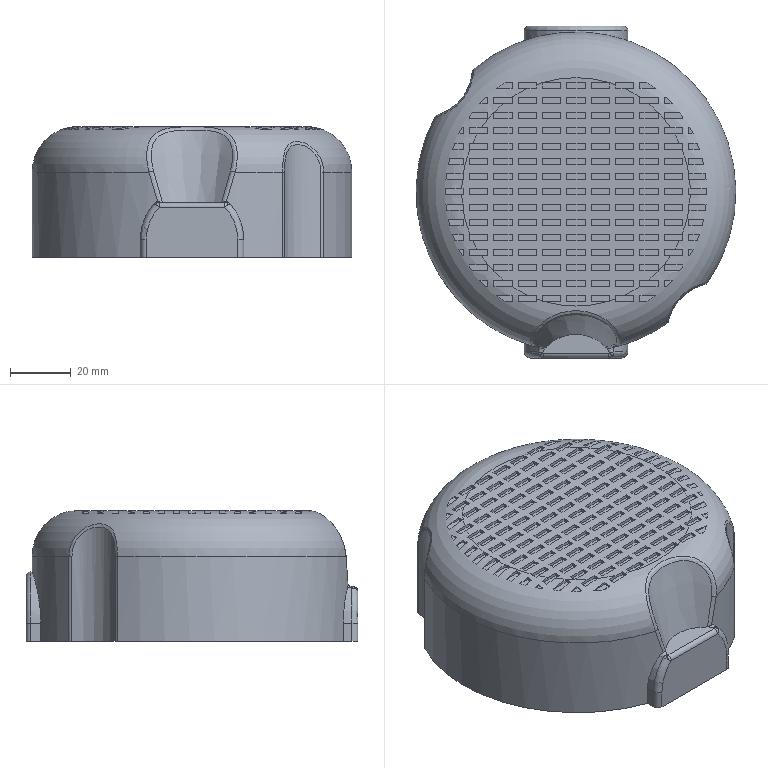Part | STEP file | CMT7E v7 | 1 solid | 763 faces | box 105 x 109 x 43 mm | volume 352834 mm3 | plane 728 | cylinder 17 | spline 13 | torus 4 | cone 1 | commonest cylinder face diameters 3 x7 34 x3 105 x3 4 x2 32 x1 33 x1